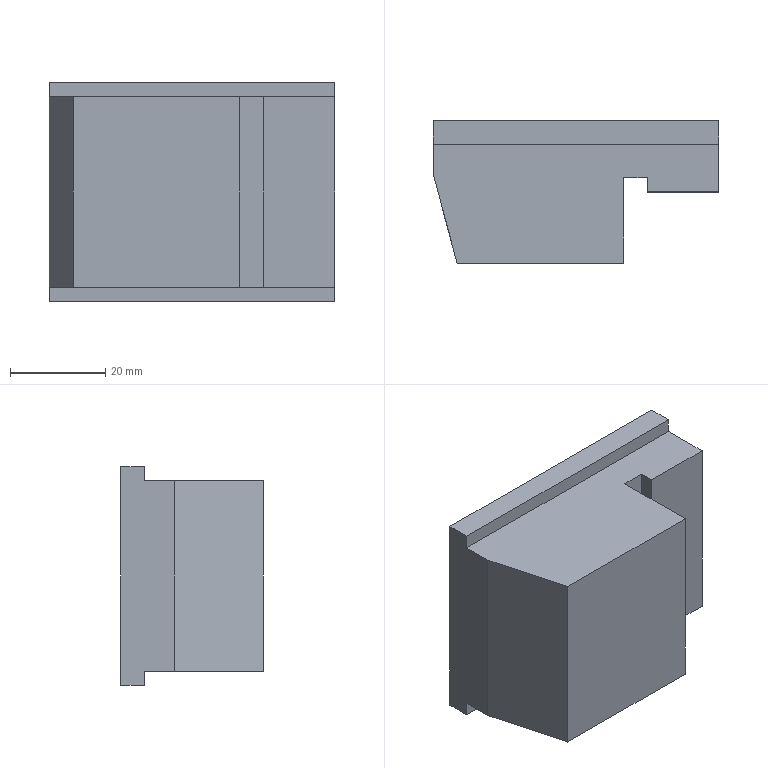Part | STEP file | 1 solid | 15 faces | box 60 x 30 x 46 mm | volume 59329 mm3 | plane 15
STEP:
#1=CARTESIAN_POINT('',(0.,0.,0.));
#2=DIRECTION('',(0.,0.,1.));
#3=DIRECTION('',(1.,0.,0.));
#4=AXIS2_PLACEMENT_3D('',#1,#2,#3);
#5=CARTESIAN_POINT('',(-197.863,83.5,180.451));
#6=VERTEX_POINT('',#5);
#7=CARTESIAN_POINT('',(-202.863,83.5,180.451));
#8=VERTEX_POINT('',#7);
#9=CARTESIAN_POINT('',(-192.81,83.5,180.451));
#10=DIRECTION('',(-1.,0.,0.));
#11=VECTOR('',#10,1.);
#12=LINE('',#9,#11);
#13=CARTESIAN_POINT('',(-192.81,69.939,180.451));
#14=DIRECTION('',(0.,0.,1.));
#15=DIRECTION('',(1.,0.,0.));
#16=AXIS2_PLACEMENT_3D('',#13,#14,#15);
#17=PLANE('',#16);
#18=CARTESIAN_POINT('',(0.,13.561));
#19=DIRECTION('',(-1.,0.));
#20=VECTOR('',#19,1.);
#21=LINE('',#18,#20);
#22=(GEOMETRIC_REPRESENTATION_CONTEXT(2)PARAMETRIC_REPRESENTATION_CONTEXT()REPRESENTATION_CONTEXT('',''));
#23=DEFINITIONAL_REPRESENTATION('',(#21),#22);
#24=PCURVE('',#17,#23);
#25=CARTESIAN_POINT('',(-161.228,83.5,160.451));
#26=DIRECTION('',(0.,1.,0.));
#27=DIRECTION('',(0.,0.,1.));
#28=AXIS2_PLACEMENT_3D('',#25,#26,#27);
#29=PLANE('',#28);
#30=CARTESIAN_POINT('',(20.,-31.582));
#31=DIRECTION('',(0.,-1.));
#32=VECTOR('',#31,1.);
#33=LINE('',#30,#32);
#34=(GEOMETRIC_REPRESENTATION_CONTEXT(2)PARAMETRIC_REPRESENTATION_CONTEXT()REPRESENTATION_CONTEXT('',''));
#35=DEFINITIONAL_REPRESENTATION('',(#33),#34);
#36=PCURVE('',#29,#35);
#37=SURFACE_CURVE('',#12,(#24,#36),.PCURVE_S1.);
#38=EDGE_CURVE('',#6,#8,#37,.T.);
#39=ORIENTED_EDGE('',*,*,#38,.F.);
#40=CARTESIAN_POINT('',(-197.863,80.5,180.451));
#41=VERTEX_POINT('',#40);
#42=CARTESIAN_POINT('',(-197.863,69.939,180.451));
#43=DIRECTION('',(0.,-1.,0.));
#44=VECTOR('',#43,1.);
#45=LINE('',#42,#44);
#46=CARTESIAN_POINT('',(-5.052,0.));
#47=DIRECTION('',(0.,-1.));
#48=VECTOR('',#47,1.);
#49=LINE('',#46,#48);
#50=(GEOMETRIC_REPRESENTATION_CONTEXT(2)PARAMETRIC_REPRESENTATION_CONTEXT()REPRESENTATION_CONTEXT('',''));
#51=DEFINITIONAL_REPRESENTATION('',(#49),#50);
#52=PCURVE('',#17,#51);
#53=CARTESIAN_POINT('',(-197.863,73.,160.451));
#54=DIRECTION('',(-1.,0.,0.));
#55=DIRECTION('',(0.,0.,1.));
#56=AXIS2_PLACEMENT_3D('',#53,#54,#55);
#57=PLANE('',#56);
#58=CARTESIAN_POINT('',(20.,-3.061));
#59=DIRECTION('',(0.,-1.));
#60=VECTOR('',#59,1.);
#61=LINE('',#58,#60);
#62=(GEOMETRIC_REPRESENTATION_CONTEXT(2)PARAMETRIC_REPRESENTATION_CONTEXT()REPRESENTATION_CONTEXT('',''));
#63=DEFINITIONAL_REPRESENTATION('',(#61),#62);
#64=PCURVE('',#57,#63);
#65=SURFACE_CURVE('',#45,(#52,#64),.PCURVE_S1.);
#66=EDGE_CURVE('',#6,#41,#65,.T.);
#67=ORIENTED_EDGE('',*,*,#66,.T.);
#68=CARTESIAN_POINT('',(-182.863,80.5,180.451));
#69=VERTEX_POINT('',#68);
#70=CARTESIAN_POINT('',(-192.81,80.5,180.451));
#71=DIRECTION('',(-1.,0.,0.));
#72=VECTOR('',#71,1.);
#73=LINE('',#70,#72);
#74=CARTESIAN_POINT('',(0.,10.561));
#75=DIRECTION('',(-1.,0.));
#76=VECTOR('',#75,1.);
#77=LINE('',#74,#76);
#78=(GEOMETRIC_REPRESENTATION_CONTEXT(2)PARAMETRIC_REPRESENTATION_CONTEXT()REPRESENTATION_CONTEXT('',''));
#79=DEFINITIONAL_REPRESENTATION('',(#77),#78);
#80=PCURVE('',#17,#79);
#81=CARTESIAN_POINT('',(-161.228,80.5,160.451));
#82=DIRECTION('',(0.,1.,0.));
#83=DIRECTION('',(0.,0.,1.));
#84=AXIS2_PLACEMENT_3D('',#81,#82,#83);
#85=PLANE('',#84);
#86=CARTESIAN_POINT('',(20.,-31.582));
#87=DIRECTION('',(0.,-1.));
#88=VECTOR('',#87,1.);
#89=LINE('',#86,#88);
#90=(GEOMETRIC_REPRESENTATION_CONTEXT(2)PARAMETRIC_REPRESENTATION_CONTEXT()REPRESENTATION_CONTEXT('',''));
#91=DEFINITIONAL_REPRESENTATION('',(#89),#90);
#92=PCURVE('',#85,#91);
#93=SURFACE_CURVE('',#73,(#80,#92),.PCURVE_S1.);
#94=EDGE_CURVE('',#69,#41,#93,.T.);
#95=ORIENTED_EDGE('',*,*,#94,.F.);
#96=CARTESIAN_POINT('',(-182.863,90.5,180.451));
#97=VERTEX_POINT('',#96);
#98=CARTESIAN_POINT('',(-182.863,90.366,180.451));
#99=DIRECTION('',(0.,1.,0.));
#100=VECTOR('',#99,1.);
#101=LINE('',#98,#100);
#102=CARTESIAN_POINT('',(9.948,20.427));
#103=DIRECTION('',(0.,1.));
#104=VECTOR('',#103,1.);
#105=LINE('',#102,#104);
#106=(GEOMETRIC_REPRESENTATION_CONTEXT(2)PARAMETRIC_REPRESENTATION_CONTEXT()REPRESENTATION_CONTEXT('',''));
#107=DEFINITIONAL_REPRESENTATION('',(#105),#106);
#108=PCURVE('',#17,#107);
#109=CARTESIAN_POINT('',(-182.863,90.366,108.53));
#110=DIRECTION('',(1.,0.,0.));
#111=DIRECTION('',(0.,0.,-1.));
#112=AXIS2_PLACEMENT_3D('',#109,#110,#111);
#113=PLANE('',#112);
#114=CARTESIAN_POINT('',(-71.922,0.));
#115=DIRECTION('',(0.,1.));
#116=VECTOR('',#115,1.);
#117=LINE('',#114,#116);
#118=(GEOMETRIC_REPRESENTATION_CONTEXT(2)PARAMETRIC_REPRESENTATION_CONTEXT()REPRESENTATION_CONTEXT('',''));
#119=DEFINITIONAL_REPRESENTATION('',(#117),#118);
#120=PCURVE('',#113,#119);
#121=SURFACE_CURVE('',#101,(#108,#120),.PCURVE_S1.);
#122=EDGE_CURVE('',#69,#97,#121,.T.);
#123=ORIENTED_EDGE('',*,*,#122,.T.);
#124=CARTESIAN_POINT('',(-242.863,90.5,180.451));
#125=VERTEX_POINT('',#124);
#126=CARTESIAN_POINT('',(-192.81,90.5,180.451));
#127=DIRECTION('',(-1.,0.,0.));
#128=VECTOR('',#127,1.);
#129=LINE('',#126,#128);
#130=CARTESIAN_POINT('',(0.,20.561));
#131=DIRECTION('',(-1.,0.));
#132=VECTOR('',#131,1.);
#133=LINE('',#130,#132);
#134=(GEOMETRIC_REPRESENTATION_CONTEXT(2)PARAMETRIC_REPRESENTATION_CONTEXT()REPRESENTATION_CONTEXT('',''));
#135=DEFINITIONAL_REPRESENTATION('',(#133),#134);
#136=PCURVE('',#17,#135);
#137=CARTESIAN_POINT('',(-207.863,90.5,160.451));
#138=DIRECTION('',(0.,1.,0.));
#139=DIRECTION('',(0.,0.,1.));
#140=AXIS2_PLACEMENT_3D('',#137,#138,#139);
#141=PLANE('',#140);
#142=CARTESIAN_POINT('',(20.,15.052));
#143=DIRECTION('',(0.,-1.));
#144=VECTOR('',#143,1.);
#145=LINE('',#142,#144);
#146=(GEOMETRIC_REPRESENTATION_CONTEXT(2)PARAMETRIC_REPRESENTATION_CONTEXT()REPRESENTATION_CONTEXT('',''));
#147=DEFINITIONAL_REPRESENTATION('',(#145),#146);
#148=PCURVE('',#141,#147);
#149=SURFACE_CURVE('',#129,(#136,#148),.PCURVE_S1.);
#150=EDGE_CURVE('',#97,#125,#149,.T.);
#151=ORIENTED_EDGE('',*,*,#150,.T.);
#152=CARTESIAN_POINT('',(-242.863,84.183,180.451));
#153=VERTEX_POINT('',#152);
#154=CARTESIAN_POINT('',(-242.863,90.366,180.451));
#155=DIRECTION('',(0.,1.,0.));
#156=VECTOR('',#155,1.);
#157=LINE('',#154,#156);
#158=CARTESIAN_POINT('',(-50.052,20.427));
#159=DIRECTION('',(0.,1.));
#160=VECTOR('',#159,1.);
#161=LINE('',#158,#160);
#162=(GEOMETRIC_REPRESENTATION_CONTEXT(2)PARAMETRIC_REPRESENTATION_CONTEXT()REPRESENTATION_CONTEXT('',''));
#163=DEFINITIONAL_REPRESENTATION('',(#161),#162);
#164=PCURVE('',#17,#163);
#165=CARTESIAN_POINT('',(-242.863,90.366,108.53));
#166=DIRECTION('',(1.,0.,0.));
#167=DIRECTION('',(0.,0.,-1.));
#168=AXIS2_PLACEMENT_3D('',#165,#166,#167);
#169=PLANE('',#168);
#170=CARTESIAN_POINT('',(-71.922,0.));
#171=DIRECTION('',(0.,1.));
#172=VECTOR('',#171,1.);
#173=LINE('',#170,#172);
#174=(GEOMETRIC_REPRESENTATION_CONTEXT(2)PARAMETRIC_REPRESENTATION_CONTEXT()REPRESENTATION_CONTEXT('',''));
#175=DEFINITIONAL_REPRESENTATION('',(#173),#174);
#176=PCURVE('',#169,#175);
#177=SURFACE_CURVE('',#157,(#164,#176),.PCURVE_S1.);
#178=EDGE_CURVE('',#153,#125,#177,.T.);
#179=ORIENTED_EDGE('',*,*,#178,.F.);
#180=CARTESIAN_POINT('',(-237.856,65.5,180.451));
#181=VERTEX_POINT('',#180);
#182=CARTESIAN_POINT('',(-242.522,82.912,180.451));
#183=DIRECTION('',(-0.2588,0.9659,0.));
#184=VECTOR('',#183,1.);
#185=LINE('',#182,#184);
#186=CARTESIAN_POINT('',(-49.711,12.973));
#187=DIRECTION('',(-0.2588,0.9659));
#188=VECTOR('',#187,1.);
#189=LINE('',#186,#188);
#190=(GEOMETRIC_REPRESENTATION_CONTEXT(2)PARAMETRIC_REPRESENTATION_CONTEXT()REPRESENTATION_CONTEXT('',''));
#191=DEFINITIONAL_REPRESENTATION('',(#189),#190);
#192=PCURVE('',#17,#191);
#193=CARTESIAN_POINT('',(-242.522,82.912,180.451));
#194=DIRECTION('',(-0.9659,-0.2588,0.));
#195=DIRECTION('',(0.2588,-0.9659,0.));
#196=AXIS2_PLACEMENT_3D('',#193,#194,#195);
#197=PLANE('',#196);
#198=CARTESIAN_POINT('',(0.,0.));
#199=DIRECTION('',(-1.,0.));
#200=VECTOR('',#199,1.);
#201=LINE('',#198,#200);
#202=(GEOMETRIC_REPRESENTATION_CONTEXT(2)PARAMETRIC_REPRESENTATION_CONTEXT()REPRESENTATION_CONTEXT('',''));
#203=DEFINITIONAL_REPRESENTATION('',(#201),#202);
#204=PCURVE('',#197,#203);
#205=SURFACE_CURVE('',#185,(#192,#204),.PCURVE_S1.);
#206=EDGE_CURVE('',#181,#153,#205,.T.);
#207=ORIENTED_EDGE('',*,*,#206,.F.);
#208=CARTESIAN_POINT('',(-202.863,65.5,180.451));
#209=VERTEX_POINT('',#208);
#210=CARTESIAN_POINT('',(-192.81,65.5,180.451));
#211=DIRECTION('',(-1.,0.,0.));
#212=VECTOR('',#211,1.);
#213=LINE('',#210,#212);
#214=CARTESIAN_POINT('',(0.,-4.439));
#215=DIRECTION('',(-1.,0.));
#216=VECTOR('',#215,1.);
#217=LINE('',#214,#216);
#218=(GEOMETRIC_REPRESENTATION_CONTEXT(2)PARAMETRIC_REPRESENTATION_CONTEXT()REPRESENTATION_CONTEXT('',''));
#219=DEFINITIONAL_REPRESENTATION('',(#217),#218);
#220=PCURVE('',#17,#219);
#221=CARTESIAN_POINT('',(-207.863,65.5,160.451));
#222=DIRECTION('',(0.,1.,0.));
#223=DIRECTION('',(0.,0.,1.));
#224=AXIS2_PLACEMENT_3D('',#221,#222,#223);
#225=PLANE('',#224);
#226=CARTESIAN_POINT('',(20.,15.052));
#227=DIRECTION('',(0.,-1.));
#228=VECTOR('',#227,1.);
#229=LINE('',#226,#228);
#230=(GEOMETRIC_REPRESENTATION_CONTEXT(2)PARAMETRIC_REPRESENTATION_CONTEXT()REPRESENTATION_CONTEXT('',''));
#231=DEFINITIONAL_REPRESENTATION('',(#229),#230);
#232=PCURVE('',#225,#231);
#233=SURFACE_CURVE('',#213,(#220,#232),.PCURVE_S1.);
#234=EDGE_CURVE('',#209,#181,#233,.T.);
#235=ORIENTED_EDGE('',*,*,#234,.F.);
#236=CARTESIAN_POINT('',(-202.863,69.939,180.451));
#237=DIRECTION('',(0.,1.,0.));
#238=VECTOR('',#237,1.);
#239=LINE('',#236,#238);
#240=CARTESIAN_POINT('',(-10.052,0.));
#241=DIRECTION('',(0.,1.));
#242=VECTOR('',#241,1.);
#243=LINE('',#240,#242);
#244=(GEOMETRIC_REPRESENTATION_CONTEXT(2)PARAMETRIC_REPRESENTATION_CONTEXT()REPRESENTATION_CONTEXT('',''));
#245=DEFINITIONAL_REPRESENTATION('',(#243),#244);
#246=PCURVE('',#17,#245);
#247=CARTESIAN_POINT('',(-202.863,80.5,160.451));
#248=DIRECTION('',(1.,0.,0.));
#249=DIRECTION('',(0.,0.,-1.));
#250=AXIS2_PLACEMENT_3D('',#247,#248,#249);
#251=PLANE('',#250);
#252=CARTESIAN_POINT('',(-20.,-10.561));
#253=DIRECTION('',(0.,1.));
#254=VECTOR('',#253,1.);
#255=LINE('',#252,#254);
#256=(GEOMETRIC_REPRESENTATION_CONTEXT(2)PARAMETRIC_REPRESENTATION_CONTEXT()REPRESENTATION_CONTEXT('',''));
#257=DEFINITIONAL_REPRESENTATION('',(#255),#256);
#258=PCURVE('',#251,#257);
#259=SURFACE_CURVE('',#239,(#246,#258),.PCURVE_S1.);
#260=EDGE_CURVE('',#209,#8,#259,.T.);
#261=ORIENTED_EDGE('',*,*,#260,.T.);
#262=EDGE_LOOP('',(#39,#67,#95,#123,#151,#179,#207,#235,#261));
#263=FACE_BOUND('',#262,.T.);
#264=ADVANCED_FACE('',(#263),#17,.T.);
#265=CARTESIAN_POINT('',(-197.863,83.5,140.451));
#266=VERTEX_POINT('',#265);
#267=CARTESIAN_POINT('',(-197.863,80.5,140.451));
#268=VERTEX_POINT('',#267);
#269=CARTESIAN_POINT('',(-197.863,69.939,140.451));
#270=DIRECTION('',(0.,-1.,0.));
#271=VECTOR('',#270,1.);
#272=LINE('',#269,#271);
#273=CARTESIAN_POINT('',(-192.81,69.939,140.451));
#274=DIRECTION('',(0.,0.,1.));
#275=DIRECTION('',(1.,0.,0.));
#276=AXIS2_PLACEMENT_3D('',#273,#274,#275);
#277=PLANE('',#276);
#278=CARTESIAN_POINT('',(-5.052,0.));
#279=DIRECTION('',(0.,-1.));
#280=VECTOR('',#279,1.);
#281=LINE('',#278,#280);
#282=(GEOMETRIC_REPRESENTATION_CONTEXT(2)PARAMETRIC_REPRESENTATION_CONTEXT()REPRESENTATION_CONTEXT('',''));
#283=DEFINITIONAL_REPRESENTATION('',(#281),#282);
#284=PCURVE('',#277,#283);
#285=CARTESIAN_POINT('',(-20.,-3.061));
#286=DIRECTION('',(0.,-1.));
#287=VECTOR('',#286,1.);
#288=LINE('',#285,#287);
#289=(GEOMETRIC_REPRESENTATION_CONTEXT(2)PARAMETRIC_REPRESENTATION_CONTEXT()REPRESENTATION_CONTEXT('',''));
#290=DEFINITIONAL_REPRESENTATION('',(#288),#289);
#291=PCURVE('',#57,#290);
#292=SURFACE_CURVE('',#272,(#284,#291),.PCURVE_S1.);
#293=EDGE_CURVE('',#266,#268,#292,.T.);
#294=ORIENTED_EDGE('',*,*,#293,.F.);
#295=CARTESIAN_POINT('',(-202.863,83.5,140.451));
#296=VERTEX_POINT('',#295);
#297=CARTESIAN_POINT('',(-192.81,83.5,140.451));
#298=DIRECTION('',(-1.,0.,0.));
#299=VECTOR('',#298,1.);
#300=LINE('',#297,#299);
#301=CARTESIAN_POINT('',(0.,13.561));
#302=DIRECTION('',(-1.,0.));
#303=VECTOR('',#302,1.);
#304=LINE('',#301,#303);
#305=(GEOMETRIC_REPRESENTATION_CONTEXT(2)PARAMETRIC_REPRESENTATION_CONTEXT()REPRESENTATION_CONTEXT('',''));
#306=DEFINITIONAL_REPRESENTATION('',(#304),#305);
#307=PCURVE('',#277,#306);
#308=CARTESIAN_POINT('',(-20.,-31.582));
#309=DIRECTION('',(0.,-1.));
#310=VECTOR('',#309,1.);
#311=LINE('',#308,#310);
#312=(GEOMETRIC_REPRESENTATION_CONTEXT(2)PARAMETRIC_REPRESENTATION_CONTEXT()REPRESENTATION_CONTEXT('',''));
#313=DEFINITIONAL_REPRESENTATION('',(#311),#312);
#314=PCURVE('',#29,#313);
#315=SURFACE_CURVE('',#300,(#307,#314),.PCURVE_S1.);
#316=EDGE_CURVE('',#266,#296,#315,.T.);
#317=ORIENTED_EDGE('',*,*,#316,.T.);
#318=CARTESIAN_POINT('',(-202.863,65.5,140.451));
#319=VERTEX_POINT('',#318);
#320=CARTESIAN_POINT('',(-202.863,69.939,140.451));
#321=DIRECTION('',(0.,1.,0.));
#322=VECTOR('',#321,1.);
#323=LINE('',#320,#322);
#324=CARTESIAN_POINT('',(-10.052,0.));
#325=DIRECTION('',(0.,1.));
#326=VECTOR('',#325,1.);
#327=LINE('',#324,#326);
#328=(GEOMETRIC_REPRESENTATION_CONTEXT(2)PARAMETRIC_REPRESENTATION_CONTEXT()REPRESENTATION_CONTEXT('',''));
#329=DEFINITIONAL_REPRESENTATION('',(#327),#328);
#330=PCURVE('',#277,#329);
#331=CARTESIAN_POINT('',(20.,-10.561));
#332=DIRECTION('',(0.,1.));
#333=VECTOR('',#332,1.);
#334=LINE('',#331,#333);
#335=(GEOMETRIC_REPRESENTATION_CONTEXT(2)PARAMETRIC_REPRESENTATION_CONTEXT()REPRESENTATION_CONTEXT('',''));
#336=DEFINITIONAL_REPRESENTATION('',(#334),#335);
#337=PCURVE('',#251,#336);
#338=SURFACE_CURVE('',#323,(#330,#337),.PCURVE_S1.);
#339=EDGE_CURVE('',#319,#296,#338,.T.);
#340=ORIENTED_EDGE('',*,*,#339,.F.);
#341=CARTESIAN_POINT('',(-237.856,65.5,140.451));
#342=VERTEX_POINT('',#341);
#343=CARTESIAN_POINT('',(-192.81,65.5,140.451));
#344=DIRECTION('',(-1.,0.,0.));
#345=VECTOR('',#344,1.);
#346=LINE('',#343,#345);
#347=CARTESIAN_POINT('',(0.,-4.439));
#348=DIRECTION('',(-1.,0.));
#349=VECTOR('',#348,1.);
#350=LINE('',#347,#349);
#351=(GEOMETRIC_REPRESENTATION_CONTEXT(2)PARAMETRIC_REPRESENTATION_CONTEXT()REPRESENTATION_CONTEXT('',''));
#352=DEFINITIONAL_REPRESENTATION('',(#350),#351);
#353=PCURVE('',#277,#352);
#354=CARTESIAN_POINT('',(-20.,15.052));
#355=DIRECTION('',(0.,-1.));
#356=VECTOR('',#355,1.);
#357=LINE('',#354,#356);
#358=(GEOMETRIC_REPRESENTATION_CONTEXT(2)PARAMETRIC_REPRESENTATION_CONTEXT()REPRESENTATION_CONTEXT('',''));
#359=DEFINITIONAL_REPRESENTATION('',(#357),#358);
#360=PCURVE('',#225,#359);
#361=SURFACE_CURVE('',#346,(#353,#360),.PCURVE_S1.);
#362=EDGE_CURVE('',#319,#342,#361,.T.);
#363=ORIENTED_EDGE('',*,*,#362,.T.);
#364=CARTESIAN_POINT('',(-242.863,84.183,140.451));
#365=VERTEX_POINT('',#364);
#366=CARTESIAN_POINT('',(-242.522,82.912,140.451));
#367=DIRECTION('',(-0.2588,0.9659,0.));
#368=VECTOR('',#367,1.);
#369=LINE('',#366,#368);
#370=CARTESIAN_POINT('',(-49.711,12.973));
#371=DIRECTION('',(-0.2588,0.9659));
#372=VECTOR('',#371,1.);
#373=LINE('',#370,#372);
#374=(GEOMETRIC_REPRESENTATION_CONTEXT(2)PARAMETRIC_REPRESENTATION_CONTEXT()REPRESENTATION_CONTEXT('',''));
#375=DEFINITIONAL_REPRESENTATION('',(#373),#374);
#376=PCURVE('',#277,#375);
#377=CARTESIAN_POINT('',(0.,-40.));
#378=DIRECTION('',(-1.,0.));
#379=VECTOR('',#378,1.);
#380=LINE('',#377,#379);
#381=(GEOMETRIC_REPRESENTATION_CONTEXT(2)PARAMETRIC_REPRESENTATION_CONTEXT()REPRESENTATION_CONTEXT('',''));
#382=DEFINITIONAL_REPRESENTATION('',(#380),#381);
#383=PCURVE('',#197,#382);
#384=SURFACE_CURVE('',#369,(#376,#383),.PCURVE_S1.);
#385=EDGE_CURVE('',#342,#365,#384,.T.);
#386=ORIENTED_EDGE('',*,*,#385,.T.);
#387=CARTESIAN_POINT('',(-242.863,90.5,140.451));
#388=VERTEX_POINT('',#387);
#389=CARTESIAN_POINT('',(-242.863,90.366,140.451));
#390=DIRECTION('',(0.,1.,0.));
#391=VECTOR('',#390,1.);
#392=LINE('',#389,#391);
#393=CARTESIAN_POINT('',(-50.052,20.427));
#394=DIRECTION('',(0.,1.));
#395=VECTOR('',#394,1.);
#396=LINE('',#393,#395);
#397=(GEOMETRIC_REPRESENTATION_CONTEXT(2)PARAMETRIC_REPRESENTATION_CONTEXT()REPRESENTATION_CONTEXT('',''));
#398=DEFINITIONAL_REPRESENTATION('',(#396),#397);
#399=PCURVE('',#277,#398);
#400=CARTESIAN_POINT('',(-31.922,0.));
#401=DIRECTION('',(0.,1.));
#402=VECTOR('',#401,1.);
#403=LINE('',#400,#402);
#404=(GEOMETRIC_REPRESENTATION_CONTEXT(2)PARAMETRIC_REPRESENTATION_CONTEXT()REPRESENTATION_CONTEXT('',''));
#405=DEFINITIONAL_REPRESENTATION('',(#403),#404);
#406=PCURVE('',#169,#405);
#407=SURFACE_CURVE('',#392,(#399,#406),.PCURVE_S1.);
#408=EDGE_CURVE('',#365,#388,#407,.T.);
#409=ORIENTED_EDGE('',*,*,#408,.T.);
#410=CARTESIAN_POINT('',(-182.863,90.5,140.451));
#411=VERTEX_POINT('',#410);
#412=CARTESIAN_POINT('',(-192.81,90.5,140.451));
#413=DIRECTION('',(-1.,0.,0.));
#414=VECTOR('',#413,1.);
#415=LINE('',#412,#414);
#416=CARTESIAN_POINT('',(0.,20.561));
#417=DIRECTION('',(-1.,0.));
#418=VECTOR('',#417,1.);
#419=LINE('',#416,#418);
#420=(GEOMETRIC_REPRESENTATION_CONTEXT(2)PARAMETRIC_REPRESENTATION_CONTEXT()REPRESENTATION_CONTEXT('',''));
#421=DEFINITIONAL_REPRESENTATION('',(#419),#420);
#422=PCURVE('',#277,#421);
#423=CARTESIAN_POINT('',(-207.863,90.5,160.451));
#424=DIRECTION('',(0.,1.,0.));
#425=DIRECTION('',(0.,0.,1.));
#426=AXIS2_PLACEMENT_3D('',#423,#424,#425);
#427=PLANE('',#426);
#428=CARTESIAN_POINT('',(-20.,15.052));
#429=DIRECTION('',(0.,-1.));
#430=VECTOR('',#429,1.);
#431=LINE('',#428,#430);
#432=(GEOMETRIC_REPRESENTATION_CONTEXT(2)PARAMETRIC_REPRESENTATION_CONTEXT()REPRESENTATION_CONTEXT('',''));
#433=DEFINITIONAL_REPRESENTATION('',(#431),#432);
#434=PCURVE('',#427,#433);
#435=SURFACE_CURVE('',#415,(#422,#434),.PCURVE_S1.);
#436=EDGE_CURVE('',#411,#388,#435,.T.);
#437=ORIENTED_EDGE('',*,*,#436,.F.);
#438=CARTESIAN_POINT('',(-182.863,80.5,140.451));
#439=VERTEX_POINT('',#438);
#440=CARTESIAN_POINT('',(-182.863,90.366,140.451));
#441=DIRECTION('',(0.,1.,0.));
#442=VECTOR('',#441,1.);
#443=LINE('',#440,#442);
#444=CARTESIAN_POINT('',(9.948,20.427));
#445=DIRECTION('',(0.,1.));
#446=VECTOR('',#445,1.);
#447=LINE('',#444,#446);
#448=(GEOMETRIC_REPRESENTATION_CONTEXT(2)PARAMETRIC_REPRESENTATION_CONTEXT()REPRESENTATION_CONTEXT('',''));
#449=DEFINITIONAL_REPRESENTATION('',(#447),#448);
#450=PCURVE('',#277,#449);
#451=CARTESIAN_POINT('',(-31.922,0.));
#452=DIRECTION('',(0.,1.));
#453=VECTOR('',#452,1.);
#454=LINE('',#451,#453);
#455=(GEOMETRIC_REPRESENTATION_CONTEXT(2)PARAMETRIC_REPRESENTATION_CONTEXT()REPRESENTATION_CONTEXT('',''));
#456=DEFINITIONAL_REPRESENTATION('',(#454),#455);
#457=PCURVE('',#113,#456);
#458=SURFACE_CURVE('',#443,(#450,#457),.PCURVE_S1.);
#459=EDGE_CURVE('',#439,#411,#458,.T.);
#460=ORIENTED_EDGE('',*,*,#459,.F.);
#461=CARTESIAN_POINT('',(-192.81,80.5,140.451));
#462=DIRECTION('',(-1.,0.,0.));
#463=VECTOR('',#462,1.);
#464=LINE('',#461,#463);
#465=CARTESIAN_POINT('',(0.,10.561));
#466=DIRECTION('',(-1.,0.));
#467=VECTOR('',#466,1.);
#468=LINE('',#465,#467);
#469=(GEOMETRIC_REPRESENTATION_CONTEXT(2)PARAMETRIC_REPRESENTATION_CONTEXT()REPRESENTATION_CONTEXT('',''));
#470=DEFINITIONAL_REPRESENTATION('',(#468),#469);
#471=PCURVE('',#277,#470);
#472=CARTESIAN_POINT('',(-20.,-31.582));
#473=DIRECTION('',(0.,-1.));
#474=VECTOR('',#473,1.);
#475=LINE('',#472,#474);
#476=(GEOMETRIC_REPRESENTATION_CONTEXT(2)PARAMETRIC_REPRESENTATION_CONTEXT()REPRESENTATION_CONTEXT('',''));
#477=DEFINITIONAL_REPRESENTATION('',(#475),#476);
#478=PCURVE('',#85,#477);
#479=SURFACE_CURVE('',#464,(#471,#478),.PCURVE_S1.);
#480=EDGE_CURVE('',#439,#268,#479,.T.);
#481=ORIENTED_EDGE('',*,*,#480,.T.);
#482=EDGE_LOOP('',(#294,#317,#340,#363,#386,#409,#437,#460,#481));
#483=FACE_BOUND('',#482,.T.);
#484=ADVANCED_FACE('',(#483),#277,.F.);
#485=CARTESIAN_POINT('',(-197.863,80.5,160.451));
#486=DIRECTION('',(0.,0.,1.));
#487=VECTOR('',#486,1.);
#488=LINE('',#485,#487);
#489=CARTESIAN_POINT('',(0.,-36.634));
#490=DIRECTION('',(1.,0.));
#491=VECTOR('',#490,1.);
#492=LINE('',#489,#491);
#493=(GEOMETRIC_REPRESENTATION_CONTEXT(2)PARAMETRIC_REPRESENTATION_CONTEXT()REPRESENTATION_CONTEXT('',''));
#494=DEFINITIONAL_REPRESENTATION('',(#492),#493);
#495=PCURVE('',#85,#494);
#496=CARTESIAN_POINT('',(0.,7.5));
#497=DIRECTION('',(1.,0.));
#498=VECTOR('',#497,1.);
#499=LINE('',#496,#498);
#500=(GEOMETRIC_REPRESENTATION_CONTEXT(2)PARAMETRIC_REPRESENTATION_CONTEXT()REPRESENTATION_CONTEXT('',''));
#501=DEFINITIONAL_REPRESENTATION('',(#499),#500);
#502=PCURVE('',#57,#501);
#503=SURFACE_CURVE('',#488,(#495,#502),.PCURVE_S1.);
#504=EDGE_CURVE('',#268,#41,#503,.T.);
#505=ORIENTED_EDGE('',*,*,#504,.F.);
#506=ORIENTED_EDGE('',*,*,#480,.F.);
#507=CARTESIAN_POINT('',(-182.863,80.5,108.53));
#508=DIRECTION('',(0.,0.,-1.));
#509=VECTOR('',#508,1.);
#510=LINE('',#507,#509);
#511=CARTESIAN_POINT('',(-51.922,-21.634));
#512=DIRECTION('',(-1.,0.));
#513=VECTOR('',#512,1.);
#514=LINE('',#511,#513);
#515=(GEOMETRIC_REPRESENTATION_CONTEXT(2)PARAMETRIC_REPRESENTATION_CONTEXT()REPRESENTATION_CONTEXT('',''));
#516=DEFINITIONAL_REPRESENTATION('',(#514),#515);
#517=PCURVE('',#85,#516);
#518=CARTESIAN_POINT('',(0.,-9.866));
#519=DIRECTION('',(1.,0.));
#520=VECTOR('',#519,1.);
#521=LINE('',#518,#520);
#522=(GEOMETRIC_REPRESENTATION_CONTEXT(2)PARAMETRIC_REPRESENTATION_CONTEXT()REPRESENTATION_CONTEXT('',''));
#523=DEFINITIONAL_REPRESENTATION('',(#521),#522);
#524=PCURVE('',#113,#523);
#525=SURFACE_CURVE('',#510,(#517,#524),.PCURVE_S1.);
#526=EDGE_CURVE('',#69,#439,#525,.T.);
#527=ORIENTED_EDGE('',*,*,#526,.F.);
#528=ORIENTED_EDGE('',*,*,#94,.T.);
#529=EDGE_LOOP('',(#505,#506,#527,#528));
#530=FACE_BOUND('',#529,.T.);
#531=ADVANCED_FACE('',(#530),#85,.F.);
#532=ORIENTED_EDGE('',*,*,#339,.T.);
#533=CARTESIAN_POINT('',(-202.863,83.5,160.451));
#534=DIRECTION('',(0.,0.,1.));
#535=VECTOR('',#534,1.);
#536=LINE('',#533,#535);
#537=CARTESIAN_POINT('',(0.,3.));
#538=DIRECTION('',(-1.,0.));
#539=VECTOR('',#538,1.);
#540=LINE('',#537,#539);
#541=(GEOMETRIC_REPRESENTATION_CONTEXT(2)PARAMETRIC_REPRESENTATION_CONTEXT()REPRESENTATION_CONTEXT('',''));
#542=DEFINITIONAL_REPRESENTATION('',(#540),#541);
#543=PCURVE('',#251,#542);
#544=CARTESIAN_POINT('',(0.,-41.634));
#545=DIRECTION('',(1.,0.));
#546=VECTOR('',#545,1.);
#547=LINE('',#544,#546);
#548=(GEOMETRIC_REPRESENTATION_CONTEXT(2)PARAMETRIC_REPRESENTATION_CONTEXT()REPRESENTATION_CONTEXT('',''));
#549=DEFINITIONAL_REPRESENTATION('',(#547),#548);
#550=PCURVE('',#29,#549);
#551=SURFACE_CURVE('',#536,(#543,#550),.PCURVE_S1.);
#552=EDGE_CURVE('',#296,#8,#551,.T.);
#553=ORIENTED_EDGE('',*,*,#552,.T.);
#554=ORIENTED_EDGE('',*,*,#260,.F.);
#555=CARTESIAN_POINT('',(-202.863,65.5,160.451));
#556=DIRECTION('',(0.,0.,-1.));
#557=VECTOR('',#556,1.);
#558=LINE('',#555,#557);
#559=CARTESIAN_POINT('',(0.,-15.));
#560=DIRECTION('',(1.,0.));
#561=VECTOR('',#560,1.);
#562=LINE('',#559,#561);
#563=(GEOMETRIC_REPRESENTATION_CONTEXT(2)PARAMETRIC_REPRESENTATION_CONTEXT()REPRESENTATION_CONTEXT('',''));
#564=DEFINITIONAL_REPRESENTATION('',(#562),#563);
#565=PCURVE('',#251,#564);
#566=CARTESIAN_POINT('',(0.,5.));
#567=DIRECTION('',(-1.,0.));
#568=VECTOR('',#567,1.);
#569=LINE('',#566,#568);
#570=(GEOMETRIC_REPRESENTATION_CONTEXT(2)PARAMETRIC_REPRESENTATION_CONTEXT()REPRESENTATION_CONTEXT('',''));
#571=DEFINITIONAL_REPRESENTATION('',(#569),#570);
#572=PCURVE('',#225,#571);
#573=SURFACE_CURVE('',#558,(#565,#572),.PCURVE_S1.);
#574=EDGE_CURVE('',#209,#319,#573,.T.);
#575=ORIENTED_EDGE('',*,*,#574,.T.);
#576=EDGE_LOOP('',(#532,#553,#554,#575));
#577=FACE_BOUND('',#576,.T.);
#578=ADVANCED_FACE('',(#577),#251,.T.);
#579=CARTESIAN_POINT('',(-182.863,90.5,137.451));
#580=VERTEX_POINT('',#579);
#581=CARTESIAN_POINT('',(-242.863,90.5,137.451));
#582=VERTEX_POINT('',#581);
#583=CARTESIAN_POINT('',(-192.81,90.5,137.451));
#584=DIRECTION('',(-1.,0.,0.));
#585=VECTOR('',#584,1.);
#586=LINE('',#583,#585);
#587=CARTESIAN_POINT('',(-23.,15.052));
#588=DIRECTION('',(0.,-1.));
#589=VECTOR('',#588,1.);
#590=LINE('',#587,#589);
#591=(GEOMETRIC_REPRESENTATION_CONTEXT(2)PARAMETRIC_REPRESENTATION_CONTEXT()REPRESENTATION_CONTEXT('',''));
#592=DEFINITIONAL_REPRESENTATION('',(#590),#591);
#593=PCURVE('',#427,#592);
#594=CARTESIAN_POINT('',(-192.81,69.939,137.451));
#595=DIRECTION('',(0.,0.,1.));
#596=DIRECTION('',(1.,0.,0.));
#597=AXIS2_PLACEMENT_3D('',#594,#595,#596);
#598=PLANE('',#597);
#599=CARTESIAN_POINT('',(0.,20.561));
#600=DIRECTION('',(-1.,0.));
#601=VECTOR('',#600,1.);
#602=LINE('',#599,#601);
#603=(GEOMETRIC_REPRESENTATION_CONTEXT(2)PARAMETRIC_REPRESENTATION_CONTEXT()REPRESENTATION_CONTEXT('',''));
#604=DEFINITIONAL_REPRESENTATION('',(#602),#603);
#605=PCURVE('',#598,#604);
#606=SURFACE_CURVE('',#586,(#593,#605),.PCURVE_S1.);
#607=EDGE_CURVE('',#580,#582,#606,.T.);
#608=ORIENTED_EDGE('',*,*,#607,.F.);
#609=CARTESIAN_POINT('',(-182.863,90.5,108.53));
#610=DIRECTION('',(0.,0.,-1.));
#611=VECTOR('',#610,1.);
#612=LINE('',#609,#611);
#613=CARTESIAN_POINT('',(-51.922,25.));
#614=DIRECTION('',(-1.,0.));
#615=VECTOR('',#614,1.);
#616=LINE('',#613,#615);
#617=(GEOMETRIC_REPRESENTATION_CONTEXT(2)PARAMETRIC_REPRESENTATION_CONTEXT()REPRESENTATION_CONTEXT('',''));
#618=DEFINITIONAL_REPRESENTATION('',(#616),#617);
#619=PCURVE('',#427,#618);
#620=CARTESIAN_POINT('',(0.,0.134));
#621=DIRECTION('',(1.,0.));
#622=VECTOR('',#621,1.);
#623=LINE('',#620,#622);
#624=(GEOMETRIC_REPRESENTATION_CONTEXT(2)PARAMETRIC_REPRESENTATION_CONTEXT()REPRESENTATION_CONTEXT('',''));
#625=DEFINITIONAL_REPRESENTATION('',(#623),#624);
#626=PCURVE('',#113,#625);
#627=SURFACE_CURVE('',#612,(#619,#626),.PCURVE_S1.);
#628=EDGE_CURVE('',#411,#580,#627,.T.);
#629=ORIENTED_EDGE('',*,*,#628,.F.);
#630=ORIENTED_EDGE('',*,*,#436,.T.);
#631=CARTESIAN_POINT('',(-242.863,90.5,108.53));
#632=DIRECTION('',(0.,0.,-1.));
#633=VECTOR('',#632,1.);
#634=LINE('',#631,#633);
#635=CARTESIAN_POINT('',(-51.922,-35.));
#636=DIRECTION('',(-1.,0.));
#637=VECTOR('',#636,1.);
#638=LINE('',#635,#637);
#639=(GEOMETRIC_REPRESENTATION_CONTEXT(2)PARAMETRIC_REPRESENTATION_CONTEXT()REPRESENTATION_CONTEXT('',''));
#640=DEFINITIONAL_REPRESENTATION('',(#638),#639);
#641=PCURVE('',#427,#640);
#642=CARTESIAN_POINT('',(0.,0.134));
#643=DIRECTION('',(1.,0.));
#644=VECTOR('',#643,1.);
#645=LINE('',#642,#644);
#646=(GEOMETRIC_REPRESENTATION_CONTEXT(2)PARAMETRIC_REPRESENTATION_CONTEXT()REPRESENTATION_CONTEXT('',''));
#647=DEFINITIONAL_REPRESENTATION('',(#645),#646);
#648=PCURVE('',#169,#647);
#649=SURFACE_CURVE('',#634,(#641,#648),.PCURVE_S1.);
#650=EDGE_CURVE('',#388,#582,#649,.T.);
#651=ORIENTED_EDGE('',*,*,#650,.T.);
#652=EDGE_LOOP('',(#608,#629,#630,#651));
#653=FACE_BOUND('',#652,.T.);
#654=ADVANCED_FACE('',(#653),#427,.F.);
#655=CARTESIAN_POINT('',(-182.863,95.5,183.451));
#656=VERTEX_POINT('',#655);
#657=CARTESIAN_POINT('',(-242.863,95.5,183.451));
#658=VERTEX_POINT('',#657);
#659=CARTESIAN_POINT('',(-232.863,95.5,183.451));
#660=DIRECTION('',(-1.,0.,0.));
#661=VECTOR('',#660,1.);
#662=LINE('',#659,#661);
#663=CARTESIAN_POINT('',(-232.863,95.5,108.53));
#664=DIRECTION('',(0.,-1.,0.));
#665=DIRECTION('',(0.,0.,-1.));
#666=AXIS2_PLACEMENT_3D('',#663,#664,#665);
#667=PLANE('',#666);
#668=CARTESIAN_POINT('',(-74.922,0.));
#669=DIRECTION('',(0.,-1.));
#670=VECTOR('',#669,1.);
#671=LINE('',#668,#670);
#672=(GEOMETRIC_REPRESENTATION_CONTEXT(2)PARAMETRIC_REPRESENTATION_CONTEXT()REPRESENTATION_CONTEXT('',''));
#673=DEFINITIONAL_REPRESENTATION('',(#671),#672);
#674=PCURVE('',#667,#673);
#675=CARTESIAN_POINT('',(-192.81,69.939,183.451));
#676=DIRECTION('',(0.,0.,1.));
#677=DIRECTION('',(1.,0.,0.));
#678=AXIS2_PLACEMENT_3D('',#675,#676,#677);
#679=PLANE('',#678);
#680=CARTESIAN_POINT('',(-40.052,25.561));
#681=DIRECTION('',(-1.,0.));
#682=VECTOR('',#681,1.);
#683=LINE('',#680,#682);
#684=(GEOMETRIC_REPRESENTATION_CONTEXT(2)PARAMETRIC_REPRESENTATION_CONTEXT()REPRESENTATION_CONTEXT('',''));
#685=DEFINITIONAL_REPRESENTATION('',(#683),#684);
#686=PCURVE('',#679,#685);
#687=SURFACE_CURVE('',#662,(#674,#686),.PCURVE_S1.);
#688=EDGE_CURVE('',#656,#658,#687,.T.);
#689=ORIENTED_EDGE('',*,*,#688,.F.);
#690=CARTESIAN_POINT('',(-182.863,95.5,137.451));
#691=VERTEX_POINT('',#690);
#692=CARTESIAN_POINT('',(-182.863,95.5,108.53));
#693=DIRECTION('',(0.,0.,-1.));
#694=VECTOR('',#693,1.);
#695=LINE('',#692,#694);
#696=CARTESIAN_POINT('',(0.,50.));
#697=DIRECTION('',(1.,0.));
#698=VECTOR('',#697,1.);
#699=LINE('',#696,#698);
#700=(GEOMETRIC_REPRESENTATION_CONTEXT(2)PARAMETRIC_REPRESENTATION_CONTEXT()REPRESENTATION_CONTEXT('',''));
#701=DEFINITIONAL_REPRESENTATION('',(#699),#700);
#702=PCURVE('',#667,#701);
#703=CARTESIAN_POINT('',(0.,5.134));
#704=DIRECTION('',(1.,0.));
#705=VECTOR('',#704,1.);
#706=LINE('',#703,#705);
#707=(GEOMETRIC_REPRESENTATION_CONTEXT(2)PARAMETRIC_REPRESENTATION_CONTEXT()REPRESENTATION_CONTEXT('',''));
#708=DEFINITIONAL_REPRESENTATION('',(#706),#707);
#709=PCURVE('',#113,#708);
#710=SURFACE_CURVE('',#695,(#702,#709),.PCURVE_S1.);
#711=EDGE_CURVE('',#656,#691,#710,.T.);
#712=ORIENTED_EDGE('',*,*,#711,.T.);
#713=CARTESIAN_POINT('',(-242.863,95.5,137.451));
#714=VERTEX_POINT('',#713);
#715=CARTESIAN_POINT('',(-232.863,95.5,137.451));
#716=DIRECTION('',(-1.,0.,0.));
#717=VECTOR('',#716,1.);
#718=LINE('',#715,#717);
#719=CARTESIAN_POINT('',(-28.922,0.));
#720=DIRECTION('',(0.,-1.));
#721=VECTOR('',#720,1.);
#722=LINE('',#719,#721);
#723=(GEOMETRIC_REPRESENTATION_CONTEXT(2)PARAMETRIC_REPRESENTATION_CONTEXT()REPRESENTATION_CONTEXT('',''));
#724=DEFINITIONAL_REPRESENTATION('',(#722),#723);
#725=PCURVE('',#667,#724);
#726=CARTESIAN_POINT('',(-40.052,25.561));
#727=DIRECTION('',(-1.,0.));
#728=VECTOR('',#727,1.);
#729=LINE('',#726,#728);
#730=(GEOMETRIC_REPRESENTATION_CONTEXT(2)PARAMETRIC_REPRESENTATION_CONTEXT()REPRESENTATION_CONTEXT('',''));
#731=DEFINITIONAL_REPRESENTATION('',(#729),#730);
#732=PCURVE('',#598,#731);
#733=SURFACE_CURVE('',#718,(#725,#732),.PCURVE_S1.);
#734=EDGE_CURVE('',#691,#714,#733,.T.);
#735=ORIENTED_EDGE('',*,*,#734,.T.);
#736=CARTESIAN_POINT('',(-242.863,95.5,108.53));
#737=DIRECTION('',(0.,0.,-1.));
#738=VECTOR('',#737,1.);
#739=LINE('',#736,#738);
#740=CARTESIAN_POINT('',(0.,-10.));
#741=DIRECTION('',(1.,0.));
#742=VECTOR('',#741,1.);
#743=LINE('',#740,#742);
#744=(GEOMETRIC_REPRESENTATION_CONTEXT(2)PARAMETRIC_REPRESENTATION_CONTEXT()REPRESENTATION_CONTEXT('',''));
#745=DEFINITIONAL_REPRESENTATION('',(#743),#744);
#746=PCURVE('',#667,#745);
#747=CARTESIAN_POINT('',(0.,5.134));
#748=DIRECTION('',(1.,0.));
#749=VECTOR('',#748,1.);
#750=LINE('',#747,#749);
#751=(GEOMETRIC_REPRESENTATION_CONTEXT(2)PARAMETRIC_REPRESENTATION_CONTEXT()REPRESENTATION_CONTEXT('',''));
#752=DEFINITIONAL_REPRESENTATION('',(#750),#751);
#753=PCURVE('',#169,#752);
#754=SURFACE_CURVE('',#739,(#746,#753),.PCURVE_S1.);
#755=EDGE_CURVE('',#658,#714,#754,.T.);
#756=ORIENTED_EDGE('',*,*,#755,.F.);
#757=EDGE_LOOP('',(#689,#712,#735,#756));
#758=FACE_BOUND('',#757,.T.);
#759=ADVANCED_FACE('',(#758),#667,.F.);
#760=ORIENTED_EDGE('',*,*,#734,.F.);
#761=CARTESIAN_POINT('',(-182.863,90.366,137.451));
#762=DIRECTION('',(0.,1.,0.));
#763=VECTOR('',#762,1.);
#764=LINE('',#761,#763);
#765=CARTESIAN_POINT('',(9.948,20.427));
#766=DIRECTION('',(0.,1.));
#767=VECTOR('',#766,1.);
#768=LINE('',#765,#767);
#769=(GEOMETRIC_REPRESENTATION_CONTEXT(2)PARAMETRIC_REPRESENTATION_CONTEXT()REPRESENTATION_CONTEXT('',''));
#770=DEFINITIONAL_REPRESENTATION('',(#768),#769);
#771=PCURVE('',#598,#770);
#772=CARTESIAN_POINT('',(-28.922,0.));
#773=DIRECTION('',(0.,1.));
#774=VECTOR('',#773,1.);
#775=LINE('',#772,#774);
#776=(GEOMETRIC_REPRESENTATION_CONTEXT(2)PARAMETRIC_REPRESENTATION_CONTEXT()REPRESENTATION_CONTEXT('',''));
#777=DEFINITIONAL_REPRESENTATION('',(#775),#776);
#778=PCURVE('',#113,#777);
#779=SURFACE_CURVE('',#764,(#771,#778),.PCURVE_S1.);
#780=EDGE_CURVE('',#580,#691,#779,.T.);
#781=ORIENTED_EDGE('',*,*,#780,.F.);
#782=ORIENTED_EDGE('',*,*,#607,.T.);
#783=CARTESIAN_POINT('',(-242.863,90.366,137.451));
#784=DIRECTION('',(0.,1.,0.));
#785=VECTOR('',#784,1.);
#786=LINE('',#783,#785);
#787=CARTESIAN_POINT('',(-50.052,20.427));
#788=DIRECTION('',(0.,1.));
#789=VECTOR('',#788,1.);
#790=LINE('',#787,#789);
#791=(GEOMETRIC_REPRESENTATION_CONTEXT(2)PARAMETRIC_REPRESENTATION_CONTEXT()REPRESENTATION_CONTEXT('',''));
#792=DEFINITIONAL_REPRESENTATION('',(#790),#791);
#793=PCURVE('',#598,#792);
#794=CARTESIAN_POINT('',(-28.922,0.));
#795=DIRECTION('',(0.,1.));
#796=VECTOR('',#795,1.);
#797=LINE('',#794,#796);
#798=(GEOMETRIC_REPRESENTATION_CONTEXT(2)PARAMETRIC_REPRESENTATION_CONTEXT()REPRESENTATION_CONTEXT('',''));
#799=DEFINITIONAL_REPRESENTATION('',(#797),#798);
#800=PCURVE('',#169,#799);
#801=SURFACE_CURVE('',#786,(#793,#800),.PCURVE_S1.);
#802=EDGE_CURVE('',#582,#714,#801,.T.);
#803=ORIENTED_EDGE('',*,*,#802,.T.);
#804=EDGE_LOOP('',(#760,#781,#782,#803));
#805=FACE_BOUND('',#804,.T.);
#806=ADVANCED_FACE('',(#805),#598,.F.);
#807=CARTESIAN_POINT('',(-182.863,90.5,183.451));
#808=VERTEX_POINT('',#807);
#809=CARTESIAN_POINT('',(-242.863,90.5,183.451));
#810=VERTEX_POINT('',#809);
#811=CARTESIAN_POINT('',(-192.81,90.5,183.451));
#812=DIRECTION('',(-1.,0.,0.));
#813=VECTOR('',#812,1.);
#814=LINE('',#811,#813);
#815=CARTESIAN_POINT('',(0.,20.561));
#816=DIRECTION('',(-1.,0.));
#817=VECTOR('',#816,1.);
#818=LINE('',#815,#817);
#819=(GEOMETRIC_REPRESENTATION_CONTEXT(2)PARAMETRIC_REPRESENTATION_CONTEXT()REPRESENTATION_CONTEXT('',''));
#820=DEFINITIONAL_REPRESENTATION('',(#818),#819);
#821=PCURVE('',#679,#820);
#822=CARTESIAN_POINT('',(23.,15.052));
#823=DIRECTION('',(0.,-1.));
#824=VECTOR('',#823,1.);
#825=LINE('',#822,#824);
#826=(GEOMETRIC_REPRESENTATION_CONTEXT(2)PARAMETRIC_REPRESENTATION_CONTEXT()REPRESENTATION_CONTEXT('',''));
#827=DEFINITIONAL_REPRESENTATION('',(#825),#826);
#828=PCURVE('',#141,#827);
#829=SURFACE_CURVE('',#814,(#821,#828),.PCURVE_S1.);
#830=EDGE_CURVE('',#808,#810,#829,.T.);
#831=ORIENTED_EDGE('',*,*,#830,.F.);
#832=CARTESIAN_POINT('',(-182.863,90.366,183.451));
#833=DIRECTION('',(0.,1.,0.));
#834=VECTOR('',#833,1.);
#835=LINE('',#832,#834);
#836=CARTESIAN_POINT('',(9.948,20.427));
#837=DIRECTION('',(0.,1.));
#838=VECTOR('',#837,1.);
#839=LINE('',#836,#838);
#840=(GEOMETRIC_REPRESENTATION_CONTEXT(2)PARAMETRIC_REPRESENTATION_CONTEXT()REPRESENTATION_CONTEXT('',''));
#841=DEFINITIONAL_REPRESENTATION('',(#839),#840);
#842=PCURVE('',#679,#841);
#843=CARTESIAN_POINT('',(-74.922,0.));
#844=DIRECTION('',(0.,1.));
#845=VECTOR('',#844,1.);
#846=LINE('',#843,#845);
#847=(GEOMETRIC_REPRESENTATION_CONTEXT(2)PARAMETRIC_REPRESENTATION_CONTEXT()REPRESENTATION_CONTEXT('',''));
#848=DEFINITIONAL_REPRESENTATION('',(#846),#847);
#849=PCURVE('',#113,#848);
#850=SURFACE_CURVE('',#835,(#842,#849),.PCURVE_S1.);
#851=EDGE_CURVE('',#808,#656,#850,.T.);
#852=ORIENTED_EDGE('',*,*,#851,.T.);
#853=ORIENTED_EDGE('',*,*,#688,.T.);
#854=CARTESIAN_POINT('',(-242.863,90.366,183.451));
#855=DIRECTION('',(0.,1.,0.));
#856=VECTOR('',#855,1.);
#857=LINE('',#854,#856);
#858=CARTESIAN_POINT('',(-50.052,20.427));
#859=DIRECTION('',(0.,1.));
#860=VECTOR('',#859,1.);
#861=LINE('',#858,#860);
#862=(GEOMETRIC_REPRESENTATION_CONTEXT(2)PARAMETRIC_REPRESENTATION_CONTEXT()REPRESENTATION_CONTEXT('',''));
#863=DEFINITIONAL_REPRESENTATION('',(#861),#862);
#864=PCURVE('',#679,#863);
#865=CARTESIAN_POINT('',(-74.922,0.));
#866=DIRECTION('',(0.,1.));
#867=VECTOR('',#866,1.);
#868=LINE('',#865,#867);
#869=(GEOMETRIC_REPRESENTATION_CONTEXT(2)PARAMETRIC_REPRESENTATION_CONTEXT()REPRESENTATION_CONTEXT('',''));
#870=DEFINITIONAL_REPRESENTATION('',(#868),#869);
#871=PCURVE('',#169,#870);
#872=SURFACE_CURVE('',#857,(#864,#871),.PCURVE_S1.);
#873=EDGE_CURVE('',#810,#658,#872,.T.);
#874=ORIENTED_EDGE('',*,*,#873,.F.);
#875=EDGE_LOOP('',(#831,#852,#853,#874));
#876=FACE_BOUND('',#875,.T.);
#877=ADVANCED_FACE('',(#876),#679,.T.);
#878=ORIENTED_EDGE('',*,*,#150,.F.);
#879=CARTESIAN_POINT('',(-182.863,90.5,108.53));
#880=DIRECTION('',(0.,0.,-1.));
#881=VECTOR('',#880,1.);
#882=LINE('',#879,#881);
#883=CARTESIAN_POINT('',(-51.922,25.));
#884=DIRECTION('',(-1.,0.));
#885=VECTOR('',#884,1.);
#886=LINE('',#883,#885);
#887=(GEOMETRIC_REPRESENTATION_CONTEXT(2)PARAMETRIC_REPRESENTATION_CONTEXT()REPRESENTATION_CONTEXT('',''));
#888=DEFINITIONAL_REPRESENTATION('',(#886),#887);
#889=PCURVE('',#141,#888);
#890=CARTESIAN_POINT('',(0.,0.134));
#891=DIRECTION('',(1.,0.));
#892=VECTOR('',#891,1.);
#893=LINE('',#890,#892);
#894=(GEOMETRIC_REPRESENTATION_CONTEXT(2)PARAMETRIC_REPRESENTATION_CONTEXT()REPRESENTATION_CONTEXT('',''));
#895=DEFINITIONAL_REPRESENTATION('',(#893),#894);
#896=PCURVE('',#113,#895);
#897=SURFACE_CURVE('',#882,(#889,#896),.PCURVE_S1.);
#898=EDGE_CURVE('',#808,#97,#897,.T.);
#899=ORIENTED_EDGE('',*,*,#898,.F.);
#900=ORIENTED_EDGE('',*,*,#830,.T.);
#901=CARTESIAN_POINT('',(-242.863,90.5,108.53));
#902=DIRECTION('',(0.,0.,-1.));
#903=VECTOR('',#902,1.);
#904=LINE('',#901,#903);
#905=CARTESIAN_POINT('',(-51.922,-35.));
#906=DIRECTION('',(-1.,0.));
#907=VECTOR('',#906,1.);
#908=LINE('',#905,#907);
#909=(GEOMETRIC_REPRESENTATION_CONTEXT(2)PARAMETRIC_REPRESENTATION_CONTEXT()REPRESENTATION_CONTEXT('',''));
#910=DEFINITIONAL_REPRESENTATION('',(#908),#909);
#911=PCURVE('',#141,#910);
#912=CARTESIAN_POINT('',(0.,0.134));
#913=DIRECTION('',(1.,0.));
#914=VECTOR('',#913,1.);
#915=LINE('',#912,#914);
#916=(GEOMETRIC_REPRESENTATION_CONTEXT(2)PARAMETRIC_REPRESENTATION_CONTEXT()REPRESENTATION_CONTEXT('',''));
#917=DEFINITIONAL_REPRESENTATION('',(#915),#916);
#918=PCURVE('',#169,#917);
#919=SURFACE_CURVE('',#904,(#911,#918),.PCURVE_S1.);
#920=EDGE_CURVE('',#810,#125,#919,.T.);
#921=ORIENTED_EDGE('',*,*,#920,.T.);
#922=EDGE_LOOP('',(#878,#899,#900,#921));
#923=FACE_BOUND('',#922,.T.);
#924=ADVANCED_FACE('',(#923),#141,.F.);
#925=ORIENTED_EDGE('',*,*,#574,.F.);
#926=ORIENTED_EDGE('',*,*,#234,.T.);
#927=CARTESIAN_POINT('',(-237.856,65.5,180.451));
#928=DIRECTION('',(0.,0.,-1.));
#929=VECTOR('',#928,1.);
#930=LINE('',#927,#929);
#931=CARTESIAN_POINT('',(20.,-29.994));
#932=DIRECTION('',(-1.,0.));
#933=VECTOR('',#932,1.);
#934=LINE('',#931,#933);
#935=(GEOMETRIC_REPRESENTATION_CONTEXT(2)PARAMETRIC_REPRESENTATION_CONTEXT()REPRESENTATION_CONTEXT('',''));
#936=DEFINITIONAL_REPRESENTATION('',(#934),#935);
#937=PCURVE('',#225,#936);
#938=CARTESIAN_POINT('',(18.026,0.));
#939=DIRECTION('',(0.,-1.));
#940=VECTOR('',#939,1.);
#941=LINE('',#938,#940);
#942=(GEOMETRIC_REPRESENTATION_CONTEXT(2)PARAMETRIC_REPRESENTATION_CONTEXT()REPRESENTATION_CONTEXT('',''));
#943=DEFINITIONAL_REPRESENTATION('',(#941),#942);
#944=PCURVE('',#197,#943);
#945=SURFACE_CURVE('',#930,(#937,#944),.PCURVE_S1.);
#946=EDGE_CURVE('',#181,#342,#945,.T.);
#947=ORIENTED_EDGE('',*,*,#946,.T.);
#948=ORIENTED_EDGE('',*,*,#362,.F.);
#949=EDGE_LOOP('',(#925,#926,#947,#948));
#950=FACE_BOUND('',#949,.T.);
#951=ADVANCED_FACE('',(#950),#225,.F.);
#952=CARTESIAN_POINT('',(-242.863,84.183,180.451));
#953=DIRECTION('',(0.,0.,-1.));
#954=VECTOR('',#953,1.);
#955=LINE('',#952,#954);
#956=CARTESIAN_POINT('',(-71.922,-6.182));
#957=DIRECTION('',(1.,0.));
#958=VECTOR('',#957,1.);
#959=LINE('',#956,#958);
#960=(GEOMETRIC_REPRESENTATION_CONTEXT(2)PARAMETRIC_REPRESENTATION_CONTEXT()REPRESENTATION_CONTEXT('',''));
#961=DEFINITIONAL_REPRESENTATION('',(#959),#960);
#962=PCURVE('',#169,#961);
#963=CARTESIAN_POINT('',(-1.317,0.));
#964=DIRECTION('',(0.,-1.));
#965=VECTOR('',#964,1.);
#966=LINE('',#963,#965);
#967=(GEOMETRIC_REPRESENTATION_CONTEXT(2)PARAMETRIC_REPRESENTATION_CONTEXT()REPRESENTATION_CONTEXT('',''));
#968=DEFINITIONAL_REPRESENTATION('',(#966),#967);
#969=PCURVE('',#197,#968);
#970=SURFACE_CURVE('',#955,(#962,#969),.PCURVE_S1.);
#971=EDGE_CURVE('',#153,#365,#970,.T.);
#972=ORIENTED_EDGE('',*,*,#971,.F.);
#973=ORIENTED_EDGE('',*,*,#178,.T.);
#974=ORIENTED_EDGE('',*,*,#920,.F.);
#975=ORIENTED_EDGE('',*,*,#873,.T.);
#976=ORIENTED_EDGE('',*,*,#755,.T.);
#977=ORIENTED_EDGE('',*,*,#802,.F.);
#978=ORIENTED_EDGE('',*,*,#650,.F.);
#979=ORIENTED_EDGE('',*,*,#408,.F.);
#980=EDGE_LOOP('',(#972,#973,#974,#975,#976,#977,#978,#979));
#981=FACE_BOUND('',#980,.T.);
#982=ADVANCED_FACE('',(#981),#169,.F.);
#983=ORIENTED_EDGE('',*,*,#206,.T.);
#984=ORIENTED_EDGE('',*,*,#971,.T.);
#985=ORIENTED_EDGE('',*,*,#385,.F.);
#986=ORIENTED_EDGE('',*,*,#946,.F.);
#987=EDGE_LOOP('',(#983,#984,#985,#986));
#988=FACE_BOUND('',#987,.T.);
#989=ADVANCED_FACE('',(#988),#197,.T.);
#990=ORIENTED_EDGE('',*,*,#122,.F.);
#991=ORIENTED_EDGE('',*,*,#526,.T.);
#992=ORIENTED_EDGE('',*,*,#459,.T.);
#993=ORIENTED_EDGE('',*,*,#628,.T.);
#994=ORIENTED_EDGE('',*,*,#780,.T.);
#995=ORIENTED_EDGE('',*,*,#711,.F.);
#996=ORIENTED_EDGE('',*,*,#851,.F.);
#997=ORIENTED_EDGE('',*,*,#898,.T.);
#998=EDGE_LOOP('',(#990,#991,#992,#993,#994,#995,#996,#997));
#999=FACE_BOUND('',#998,.T.);
#1000=ADVANCED_FACE('',(#999),#113,.T.);
#1001=ORIENTED_EDGE('',*,*,#504,.T.);
#1002=ORIENTED_EDGE('',*,*,#66,.F.);
#1003=CARTESIAN_POINT('',(-197.863,83.5,160.451));
#1004=DIRECTION('',(0.,0.,1.));
#1005=VECTOR('',#1004,1.);
#1006=LINE('',#1003,#1005);
#1007=CARTESIAN_POINT('',(0.,10.5));
#1008=DIRECTION('',(1.,0.));
#1009=VECTOR('',#1008,1.);
#1010=LINE('',#1007,#1009);
#1011=(GEOMETRIC_REPRESENTATION_CONTEXT(2)PARAMETRIC_REPRESENTATION_CONTEXT()REPRESENTATION_CONTEXT('',''));
#1012=DEFINITIONAL_REPRESENTATION('',(#1010),#1011);
#1013=PCURVE('',#57,#1012);
#1014=CARTESIAN_POINT('',(0.,-36.634));
#1015=DIRECTION('',(1.,0.));
#1016=VECTOR('',#1015,1.);
#1017=LINE('',#1014,#1016);
#1018=(GEOMETRIC_REPRESENTATION_CONTEXT(2)PARAMETRIC_REPRESENTATION_CONTEXT()REPRESENTATION_CONTEXT('',''));
#1019=DEFINITIONAL_REPRESENTATION('',(#1017),#1018);
#1020=PCURVE('',#29,#1019);
#1021=SURFACE_CURVE('',#1006,(#1013,#1020),.PCURVE_S1.);
#1022=EDGE_CURVE('',#266,#6,#1021,.T.);
#1023=ORIENTED_EDGE('',*,*,#1022,.F.);
#1024=ORIENTED_EDGE('',*,*,#293,.T.);
#1025=EDGE_LOOP('',(#1001,#1002,#1023,#1024));
#1026=FACE_BOUND('',#1025,.T.);
#1027=ADVANCED_FACE('',(#1026),#57,.T.);
#1028=ORIENTED_EDGE('',*,*,#1022,.T.);
#1029=ORIENTED_EDGE('',*,*,#38,.T.);
#1030=ORIENTED_EDGE('',*,*,#552,.F.);
#1031=ORIENTED_EDGE('',*,*,#316,.F.);
#1032=EDGE_LOOP('',(#1028,#1029,#1030,#1031));
#1033=FACE_BOUND('',#1032,.T.);
#1034=ADVANCED_FACE('',(#1033),#29,.F.);
#1035=CLOSED_SHELL('',(#264,#484,#531,#578,#654,#759,#806,#877,#924,#951,#982,#989,#1000,#1027,#1034));
#1036=MANIFOLD_SOLID_BREP('',#1035);
#1037=(LENGTH_UNIT()NAMED_UNIT(*)SI_UNIT(.MILLI.,.METRE.));
#1038=UNCERTAINTY_MEASURE_WITH_UNIT(LENGTH_MEASURE(0.0000001),#1037,'','');
#1039=(NAMED_UNIT(*)PLANE_ANGLE_UNIT()SI_UNIT($,.RADIAN.));
#1040=(NAMED_UNIT(*)SI_UNIT($,.STERADIAN.)SOLID_ANGLE_UNIT());
#1041=(GEOMETRIC_REPRESENTATION_CONTEXT(3)GLOBAL_UNCERTAINTY_ASSIGNED_CONTEXT((#1038))GLOBAL_UNIT_ASSIGNED_CONTEXT((#1037,#1039,#1040))REPRESENTATION_CONTEXT('',''));
#1042=ADVANCED_BREP_SHAPE_REPRESENTATION('',(#4,#1036),#1041);